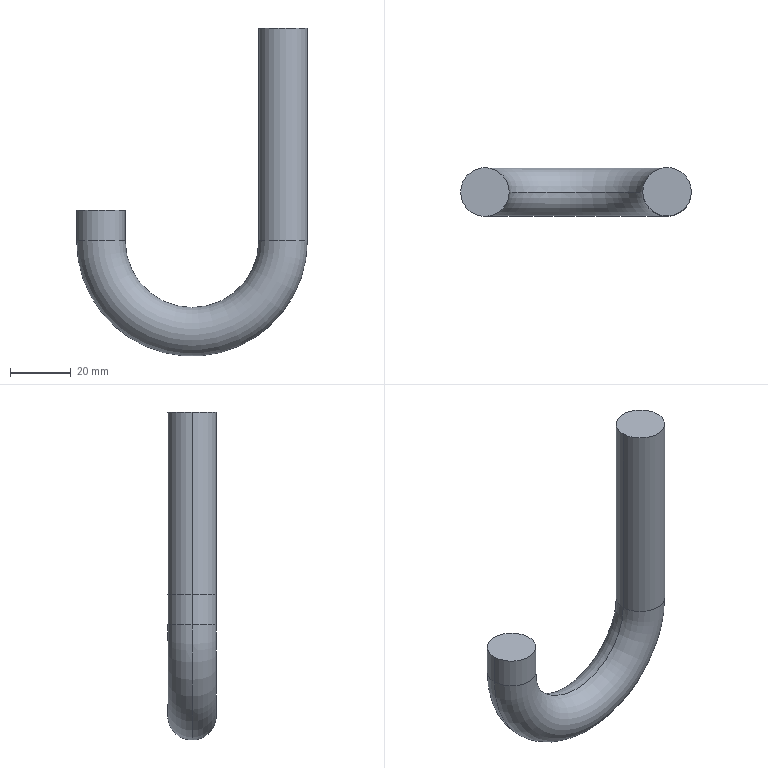Part | SolidWorks | features Sweep 1 | 1 solid | 8 faces | box 76 x 16 x 108 mm | volume 35035 mm3 | cylinder 4 | torus 2 | plane 2 | commonest cylinder face diameters 16 x4
STEP:
#1=CARTESIAN_POINT('',(8.,0.,-70.));
#2=VERTEX_POINT('',#1);
#3=CARTESIAN_POINT('',(-8.,0.,-70.));
#4=VERTEX_POINT('',#3);
#5=CARTESIAN_POINT('',(0.,0.,-70.));
#6=DIRECTION('',(0.,0.,1.));
#7=DIRECTION('',(1.,0.,0.));
#8=AXIS2_PLACEMENT_3D('',#5,#6,#7);
#9=CIRCLE('',#8,8.);
#10=EDGE_CURVE('',#2,#4,#9,.T.);
#11=ORIENTED_EDGE('',*,*,#10,.F.);
#12=CARTESIAN_POINT('',(-68.,0.,-70.));
#13=VERTEX_POINT('',#12);
#14=CARTESIAN_POINT('',(-30.,0.,-70.));
#15=DIRECTION('',(0.,1.,0.));
#16=DIRECTION('',(0.,0.,1.));
#17=AXIS2_PLACEMENT_3D('',#14,#15,#16);
#18=CIRCLE('',#17,38.);
#19=EDGE_CURVE('',#2,#13,#18,.T.);
#20=ORIENTED_EDGE('',*,*,#19,.T.);
#21=CARTESIAN_POINT('',(-52.,0.,-70.));
#22=VERTEX_POINT('',#21);
#23=CARTESIAN_POINT('',(-60.,0.,-70.));
#24=DIRECTION('',(0.,0.,-1.));
#25=DIRECTION('',(-1.,0.,0.));
#26=AXIS2_PLACEMENT_3D('',#23,#24,#25);
#27=CIRCLE('',#26,8.);
#28=EDGE_CURVE('',#13,#22,#27,.T.);
#29=ORIENTED_EDGE('',*,*,#28,.T.);
#30=CARTESIAN_POINT('',(-30.,0.,-70.));
#31=DIRECTION('',(0.,1.,0.));
#32=DIRECTION('',(0.,0.,1.));
#33=AXIS2_PLACEMENT_3D('',#30,#31,#32);
#34=CIRCLE('',#33,22.);
#35=EDGE_CURVE('',#4,#22,#34,.T.);
#36=ORIENTED_EDGE('',*,*,#35,.F.);
#37=EDGE_LOOP('',(#11,#20,#29,#36));
#38=FACE_OUTER_BOUND('',#37,.T.);
#39=CARTESIAN_POINT('',(-30.,0.,-70.));
#40=DIRECTION('',(0.,1.,0.));
#41=DIRECTION('',(0.,0.,1.));
#42=AXIS2_PLACEMENT_3D('',#39,#40,#41);
#43=TOROIDAL_SURFACE('',#42,30.,8.);
#44=ADVANCED_FACE('',(#38),#43,.T.);
#45=ORIENTED_EDGE('',*,*,#28,.F.);
#46=CARTESIAN_POINT('',(-68.,0.,-60.));
#47=VERTEX_POINT('',#46);
#48=CARTESIAN_POINT('',(-68.,0.,-70.));
#49=DIRECTION('',(0.,0.,1.));
#50=VECTOR('',#49,1000.);
#51=LINE('',#48,#50);
#52=EDGE_CURVE('',#13,#47,#51,.T.);
#53=ORIENTED_EDGE('',*,*,#52,.T.);
#54=CARTESIAN_POINT('',(-52.,0.,-60.));
#55=VERTEX_POINT('',#54);
#56=CARTESIAN_POINT('',(-60.,0.,-60.));
#57=DIRECTION('',(0.,0.,-1.));
#58=DIRECTION('',(-1.,0.,0.));
#59=AXIS2_PLACEMENT_3D('',#56,#57,#58);
#60=CIRCLE('',#59,8.);
#61=EDGE_CURVE('',#47,#55,#60,.T.);
#62=ORIENTED_EDGE('',*,*,#61,.T.);
#63=CARTESIAN_POINT('',(-52.,0.,-70.));
#64=DIRECTION('',(0.,0.,1.));
#65=VECTOR('',#64,1000.);
#66=LINE('',#63,#65);
#67=EDGE_CURVE('',#22,#55,#66,.T.);
#68=ORIENTED_EDGE('',*,*,#67,.F.);
#69=EDGE_LOOP('',(#45,#53,#62,#68));
#70=FACE_OUTER_BOUND('',#69,.T.);
#71=CARTESIAN_POINT('',(-60.,0.,-70.));
#72=DIRECTION('',(0.,0.,1.));
#73=DIRECTION('',(1.,0.,0.));
#74=AXIS2_PLACEMENT_3D('',#71,#72,#73);
#75=CYLINDRICAL_SURFACE('',#74,8.);
#76=ADVANCED_FACE('',(#70),#75,.T.);
#77=CARTESIAN_POINT('',(8.,0.,0.));
#78=VERTEX_POINT('',#77);
#79=CARTESIAN_POINT('',(-8.,0.,0.));
#80=VERTEX_POINT('',#79);
#81=CARTESIAN_POINT('',(0.,0.,0.));
#82=DIRECTION('',(0.,0.,1.));
#83=DIRECTION('',(1.,0.,0.));
#84=AXIS2_PLACEMENT_3D('',#81,#82,#83);
#85=CIRCLE('',#84,8.);
#86=EDGE_CURVE('',#78,#80,#85,.T.);
#87=ORIENTED_EDGE('',*,*,#86,.F.);
#88=CARTESIAN_POINT('',(8.,0.,0.));
#89=DIRECTION('',(0.,0.,-1.));
#90=VECTOR('',#89,1000.);
#91=LINE('',#88,#90);
#92=EDGE_CURVE('',#78,#2,#91,.T.);
#93=ORIENTED_EDGE('',*,*,#92,.T.);
#94=ORIENTED_EDGE('',*,*,#10,.T.);
#95=CARTESIAN_POINT('',(-8.,0.,0.));
#96=DIRECTION('',(0.,0.,-1.));
#97=VECTOR('',#96,1000.);
#98=LINE('',#95,#97);
#99=EDGE_CURVE('',#80,#4,#98,.T.);
#100=ORIENTED_EDGE('',*,*,#99,.F.);
#101=EDGE_LOOP('',(#87,#93,#94,#100));
#102=FACE_OUTER_BOUND('',#101,.T.);
#103=CARTESIAN_POINT('',(0.,0.,0.));
#104=DIRECTION('',(0.,0.,-1.));
#105=DIRECTION('',(-1.,0.,0.));
#106=AXIS2_PLACEMENT_3D('',#103,#104,#105);
#107=CYLINDRICAL_SURFACE('',#106,8.);
#108=ADVANCED_FACE('',(#102),#107,.T.);
#109=ORIENTED_EDGE('',*,*,#52,.F.);
#110=CARTESIAN_POINT('',(-60.,0.,-70.));
#111=DIRECTION('',(0.,0.,-1.));
#112=DIRECTION('',(-1.,0.,0.));
#113=AXIS2_PLACEMENT_3D('',#110,#111,#112);
#114=CIRCLE('',#113,8.);
#115=EDGE_CURVE('',#22,#13,#114,.T.);
#116=ORIENTED_EDGE('',*,*,#115,.F.);
#117=ORIENTED_EDGE('',*,*,#67,.T.);
#118=CARTESIAN_POINT('',(-60.,0.,-60.));
#119=DIRECTION('',(0.,0.,-1.));
#120=DIRECTION('',(-1.,0.,0.));
#121=AXIS2_PLACEMENT_3D('',#118,#119,#120);
#122=CIRCLE('',#121,8.);
#123=EDGE_CURVE('',#55,#47,#122,.T.);
#124=ORIENTED_EDGE('',*,*,#123,.T.);
#125=EDGE_LOOP('',(#109,#116,#117,#124));
#126=FACE_OUTER_BOUND('',#125,.T.);
#127=CARTESIAN_POINT('',(-60.,0.,-70.));
#128=DIRECTION('',(0.,0.,1.));
#129=DIRECTION('',(1.,0.,0.));
#130=AXIS2_PLACEMENT_3D('',#127,#128,#129);
#131=CYLINDRICAL_SURFACE('',#130,8.);
#132=ADVANCED_FACE('',(#126),#131,.T.);
#133=ORIENTED_EDGE('',*,*,#19,.F.);
#134=CARTESIAN_POINT('',(0.,0.,-70.));
#135=DIRECTION('',(0.,0.,1.));
#136=DIRECTION('',(1.,0.,0.));
#137=AXIS2_PLACEMENT_3D('',#134,#135,#136);
#138=CIRCLE('',#137,8.);
#139=EDGE_CURVE('',#4,#2,#138,.T.);
#140=ORIENTED_EDGE('',*,*,#139,.F.);
#141=ORIENTED_EDGE('',*,*,#35,.T.);
#142=ORIENTED_EDGE('',*,*,#115,.T.);
#143=EDGE_LOOP('',(#133,#140,#141,#142));
#144=FACE_OUTER_BOUND('',#143,.T.);
#145=CARTESIAN_POINT('',(-30.,0.,-70.));
#146=DIRECTION('',(0.,1.,0.));
#147=DIRECTION('',(0.,0.,1.));
#148=AXIS2_PLACEMENT_3D('',#145,#146,#147);
#149=TOROIDAL_SURFACE('',#148,30.,8.);
#150=ADVANCED_FACE('',(#144),#149,.T.);
#151=ORIENTED_EDGE('',*,*,#92,.F.);
#152=CARTESIAN_POINT('',(0.,0.,0.));
#153=DIRECTION('',(0.,0.,1.));
#154=DIRECTION('',(1.,0.,0.));
#155=AXIS2_PLACEMENT_3D('',#152,#153,#154);
#156=CIRCLE('',#155,8.);
#157=EDGE_CURVE('',#80,#78,#156,.T.);
#158=ORIENTED_EDGE('',*,*,#157,.F.);
#159=ORIENTED_EDGE('',*,*,#99,.T.);
#160=ORIENTED_EDGE('',*,*,#139,.T.);
#161=EDGE_LOOP('',(#151,#158,#159,#160));
#162=FACE_OUTER_BOUND('',#161,.T.);
#163=CARTESIAN_POINT('',(0.,0.,0.));
#164=DIRECTION('',(0.,0.,-1.));
#165=DIRECTION('',(-1.,0.,0.));
#166=AXIS2_PLACEMENT_3D('',#163,#164,#165);
#167=CYLINDRICAL_SURFACE('',#166,8.);
#168=ADVANCED_FACE('',(#162),#167,.T.);
#169=ORIENTED_EDGE('',*,*,#123,.F.);
#170=ORIENTED_EDGE('',*,*,#61,.F.);
#171=EDGE_LOOP('',(#169,#170));
#172=FACE_OUTER_BOUND('',#171,.T.);
#173=CARTESIAN_POINT('',(-60.,0.,-60.));
#174=DIRECTION('',(0.,0.,-1.));
#175=DIRECTION('',(-1.,0.,0.));
#176=AXIS2_PLACEMENT_3D('',#173,#174,#175);
#177=PLANE('',#176);
#178=ADVANCED_FACE('',(#172),#177,.F.);
#179=ORIENTED_EDGE('',*,*,#157,.T.);
#180=ORIENTED_EDGE('',*,*,#86,.T.);
#181=EDGE_LOOP('',(#179,#180));
#182=FACE_OUTER_BOUND('',#181,.T.);
#183=CARTESIAN_POINT('',(0.,0.,0.));
#184=DIRECTION('',(0.,0.,1.));
#185=DIRECTION('',(1.,0.,0.));
#186=AXIS2_PLACEMENT_3D('',#183,#184,#185);
#187=PLANE('',#186);
#188=ADVANCED_FACE('',(#182),#187,.T.);
#189=CLOSED_SHELL('',(#44,#76,#108,#132,#150,#168,#178,#188));
#190=MANIFOLD_SOLID_BREP('',#189);
#191=CARTESIAN_POINT('',(0.,0.,0.));
#192=DIRECTION('',(0.,0.,1.));
#193=DIRECTION('',(1.,0.,0.));
#194=AXIS2_PLACEMENT_3D('',#191,#192,#193);
#195=(LENGTH_UNIT()NAMED_UNIT(*)SI_UNIT(.MILLI.,.METRE.));
#196=UNCERTAINTY_MEASURE_WITH_UNIT(LENGTH_MEASURE(0.00001),#195,'','');
#197=(NAMED_UNIT(*)PLANE_ANGLE_UNIT()SI_UNIT($,.RADIAN.));
#198=(NAMED_UNIT(*)SI_UNIT($,.STERADIAN.)SOLID_ANGLE_UNIT());
#199=(GEOMETRIC_REPRESENTATION_CONTEXT(3)GLOBAL_UNCERTAINTY_ASSIGNED_CONTEXT((#196))GLOBAL_UNIT_ASSIGNED_CONTEXT((#195,#197,#198))REPRESENTATION_CONTEXT('',''));
#200=ADVANCED_BREP_SHAPE_REPRESENTATION('',(#190,#194),#199);